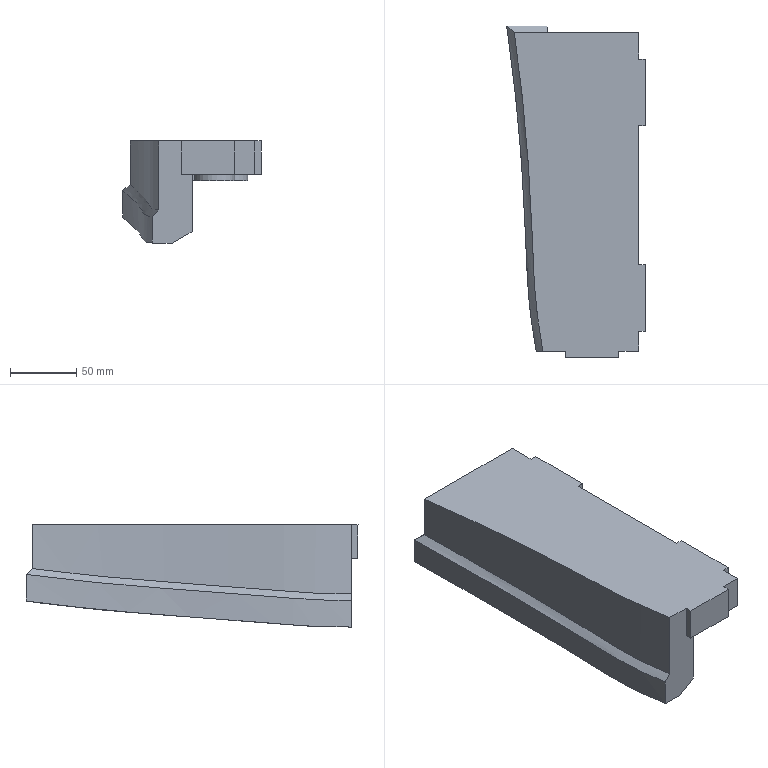Part | NX | features solid 2 | 1 solid | 35 faces | box 104.309 x 250 x 76.899 mm | volume 810856 mm3 | plane 24 | spline 6 | cylinder 5 | commonest cylinder face diameters 30 x5